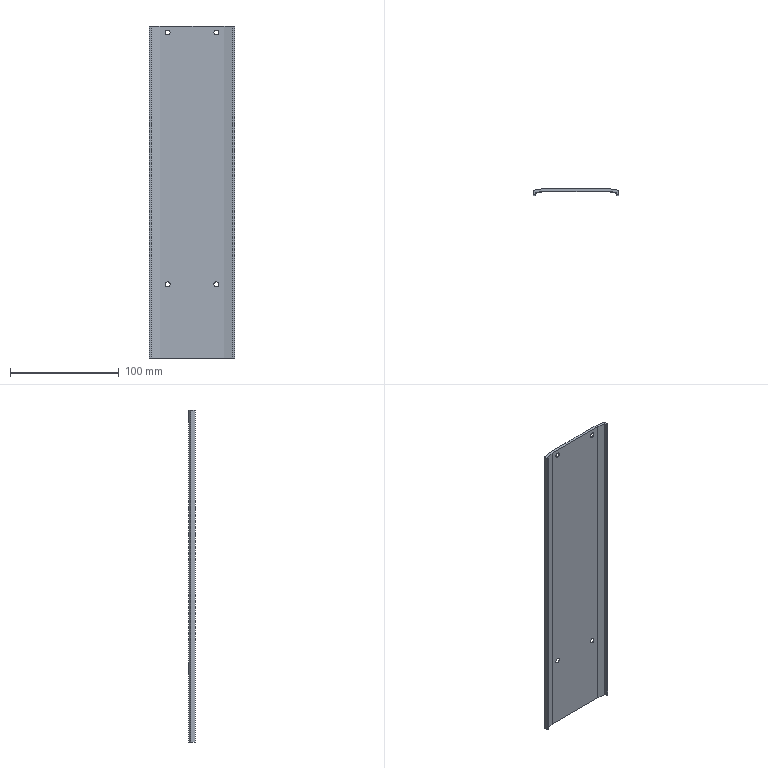Part | SolidWorks | features ICE 4, Extrusion 1, HoleWzd 1 | 1 solid | 95 faces | box 79 x 6 x 306 mm | volume 62238 mm3 | plane 61 | spline 18 | cone 8 | cylinder 8 | commonest cylinder face diameters 4.5 x8